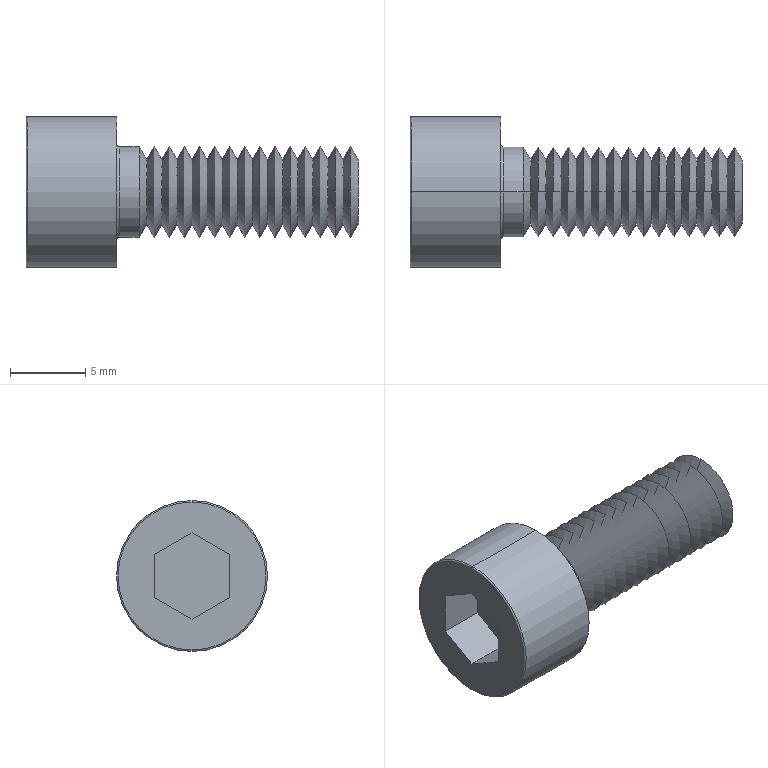Part | SolidWorks | features BlendCut 1, Cut 1, Fillet 1, LPattern 1, RevCut 1, Revolution 1 | 1 solid | 104 faces | box 22 x 10 x 10 mm | volume 753.015 mm3 | cone 58 | cylinder 32 | plane 10 | torus 4 | commonest cylinder face diameters 6 x30 10 x2